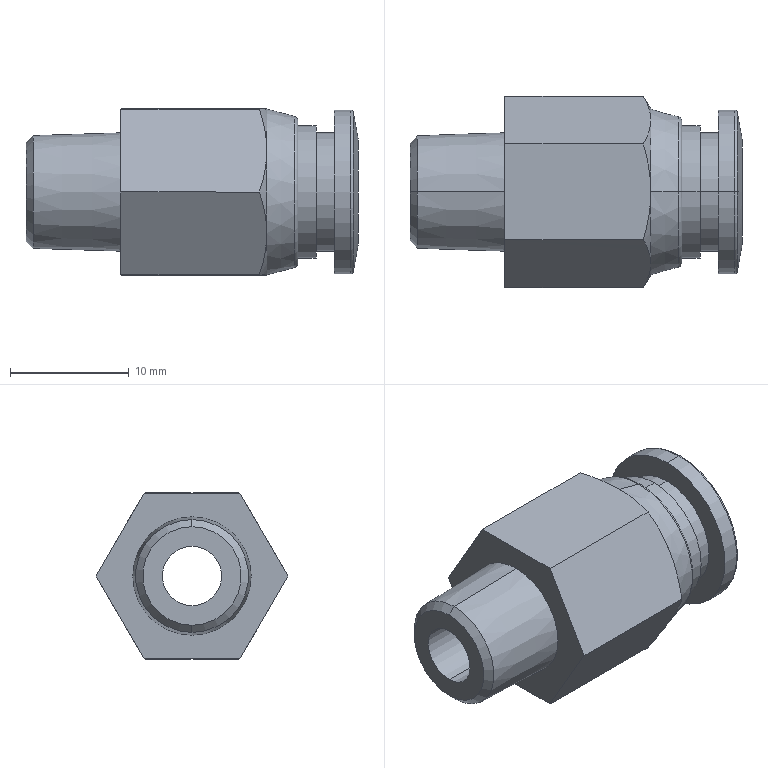Part | SolidWorks | features Fillet 2, BaseBody 1, Chamfer 1, HoleWzd 1, ICE 1, Revolution 1 | 1 solid | 41 faces | box 28 x 16.166 x 14 mm | volume 2490 mm3 | cone 14 | plane 13 | cylinder 10 | torus 4 | commonest cylinder face diameters 5 x2 8 x2 10 x2 11.2 x2 13.8 x2
STEP:
#1=CARTESIAN_POINT('',(22.923,0.,-5.992));
#2=VERTEX_POINT('',#1);
#3=CARTESIAN_POINT('',(22.923,0.,5.992));
#4=VERTEX_POINT('',#3);
#5=CARTESIAN_POINT('',(22.923,0.,0.));
#6=DIRECTION('',(1.,0.,0.));
#7=DIRECTION('',(0.,0.,1.));
#8=AXIS2_PLACEMENT_3D('',#5,#6,#7);
#9=CIRCLE('',#8,5.992);
#10=EDGE_CURVE('',#2,#4,#9,.T.);
#11=ORIENTED_EDGE('',*,*,#10,.F.);
#12=CARTESIAN_POINT('',(22.627,0.,-6.379));
#13=VERTEX_POINT('',#12);
#14=CARTESIAN_POINT('',(22.523,0.,-5.992));
#15=DIRECTION('',(0.,1.,0.));
#16=DIRECTION('',(0.,0.,1.));
#17=AXIS2_PLACEMENT_3D('',#14,#15,#16);
#18=CIRCLE('',#17,0.4);
#19=EDGE_CURVE('',#2,#13,#18,.T.);
#20=ORIENTED_EDGE('',*,*,#19,.T.);
#21=CARTESIAN_POINT('',(22.627,0.,6.379));
#22=VERTEX_POINT('',#21);
#23=CARTESIAN_POINT('',(22.627,0.,0.));
#24=DIRECTION('',(-1.,0.,0.));
#25=DIRECTION('',(0.,0.,1.));
#26=AXIS2_PLACEMENT_3D('',#23,#24,#25);
#27=CIRCLE('',#26,6.379);
#28=EDGE_CURVE('',#22,#13,#27,.T.);
#29=ORIENTED_EDGE('',*,*,#28,.F.);
#30=CARTESIAN_POINT('',(22.523,0.,5.992));
#31=DIRECTION('',(0.,-1.,0.));
#32=DIRECTION('',(1.,0.,0.));
#33=AXIS2_PLACEMENT_3D('',#30,#31,#32);
#34=CIRCLE('',#33,0.4);
#35=EDGE_CURVE('',#4,#22,#34,.T.);
#36=ORIENTED_EDGE('',*,*,#35,.F.);
#37=EDGE_LOOP('',(#11,#20,#29,#36));
#38=FACE_OUTER_BOUND('',#37,.T.);
#39=CARTESIAN_POINT('',(22.523,0.,0.));
#40=DIRECTION('',(-1.,0.,0.));
#41=DIRECTION('',(0.,0.,1.));
#42=AXIS2_PLACEMENT_3D('',#39,#40,#41);
#43=TOROIDAL_SURFACE('',#42,5.992,0.4);
#44=ADVANCED_FACE('',(#38),#43,.T.);
#45=CARTESIAN_POINT('',(27.606,0.,-6.735));
#46=VERTEX_POINT('',#45);
#47=CARTESIAN_POINT('',(27.606,0.,6.735));
#48=VERTEX_POINT('',#47);
#49=CARTESIAN_POINT('',(27.606,0.,0.));
#50=DIRECTION('',(1.,0.,0.));
#51=DIRECTION('',(0.,0.,-1.));
#52=AXIS2_PLACEMENT_3D('',#49,#50,#51);
#53=CIRCLE('',#52,6.735);
#54=EDGE_CURVE('',#46,#48,#53,.T.);
#55=ORIENTED_EDGE('',*,*,#54,.F.);
#56=CARTESIAN_POINT('',(27.409,0.,-6.9));
#57=VERTEX_POINT('',#56);
#58=CARTESIAN_POINT('',(27.409,0.,-6.7));
#59=DIRECTION('',(0.,1.,0.));
#60=DIRECTION('',(0.,0.,1.));
#61=AXIS2_PLACEMENT_3D('',#58,#59,#60);
#62=CIRCLE('',#61,0.2);
#63=EDGE_CURVE('',#46,#57,#62,.T.);
#64=ORIENTED_EDGE('',*,*,#63,.T.);
#65=CARTESIAN_POINT('',(27.409,0.,6.9));
#66=VERTEX_POINT('',#65);
#67=CARTESIAN_POINT('',(27.409,0.,0.));
#68=DIRECTION('',(-1.,0.,0.));
#69=DIRECTION('',(0.,0.,1.));
#70=AXIS2_PLACEMENT_3D('',#67,#68,#69);
#71=CIRCLE('',#70,6.9);
#72=EDGE_CURVE('',#66,#57,#71,.T.);
#73=ORIENTED_EDGE('',*,*,#72,.F.);
#74=CARTESIAN_POINT('',(27.409,0.,6.7));
#75=DIRECTION('',(0.,-1.,0.));
#76=DIRECTION('',(1.,0.,0.));
#77=AXIS2_PLACEMENT_3D('',#74,#75,#76);
#78=CIRCLE('',#77,0.2);
#79=EDGE_CURVE('',#48,#66,#78,.T.);
#80=ORIENTED_EDGE('',*,*,#79,.F.);
#81=EDGE_LOOP('',(#55,#64,#73,#80));
#82=FACE_OUTER_BOUND('',#81,.T.);
#83=CARTESIAN_POINT('',(27.409,0.,0.));
#84=DIRECTION('',(-1.,0.,0.));
#85=DIRECTION('',(0.,0.,1.));
#86=AXIS2_PLACEMENT_3D('',#83,#84,#85);
#87=TOROIDAL_SURFACE('',#86,6.7,0.2);
#88=ADVANCED_FACE('',(#82),#87,.T.);
#89=CARTESIAN_POINT('',(0.,0.,4.158));
#90=VERTEX_POINT('',#89);
#91=CARTESIAN_POINT('',(0.,0.,-4.158));
#92=VERTEX_POINT('',#91);
#93=CARTESIAN_POINT('',(0.,0.,0.));
#94=DIRECTION('',(-1.,0.,0.));
#95=DIRECTION('',(0.,0.,1.));
#96=AXIS2_PLACEMENT_3D('',#93,#94,#95);
#97=CIRCLE('',#96,4.158);
#98=EDGE_CURVE('',#90,#92,#97,.T.);
#99=ORIENTED_EDGE('',*,*,#98,.F.);
#100=CARTESIAN_POINT('',(0.5997,0.,4.758));
#101=VERTEX_POINT('',#100);
#102=CARTESIAN_POINT('',(0.,0.,4.158));
#103=DIRECTION('',(0.7071,0.,0.7071));
#104=VECTOR('',#103,1000.);
#105=LINE('',#102,#104);
#106=EDGE_CURVE('',#90,#101,#105,.T.);
#107=ORIENTED_EDGE('',*,*,#106,.T.);
#108=CARTESIAN_POINT('',(0.5997,0.,-4.758));
#109=VERTEX_POINT('',#108);
#110=CARTESIAN_POINT('',(0.5997,0.,0.));
#111=DIRECTION('',(1.,0.,0.));
#112=DIRECTION('',(0.,0.,1.));
#113=AXIS2_PLACEMENT_3D('',#110,#111,#112);
#114=CIRCLE('',#113,4.758);
#115=EDGE_CURVE('',#109,#101,#114,.T.);
#116=ORIENTED_EDGE('',*,*,#115,.F.);
#117=CARTESIAN_POINT('',(0.,0.,-4.158));
#118=DIRECTION('',(0.7071,0.,-0.7071));
#119=VECTOR('',#118,1000.);
#120=LINE('',#117,#119);
#121=EDGE_CURVE('',#92,#109,#120,.T.);
#122=ORIENTED_EDGE('',*,*,#121,.F.);
#123=EDGE_LOOP('',(#99,#107,#116,#122));
#124=FACE_OUTER_BOUND('',#123,.T.);
#125=CARTESIAN_POINT('',(0.,0.,0.));
#126=DIRECTION('',(1.,0.,0.));
#127=DIRECTION('',(0.,0.,-1.));
#128=AXIS2_PLACEMENT_3D('',#125,#126,#127);
#129=CONICAL_SURFACE('',#128,4.158,0.7854);
#130=ADVANCED_FACE('',(#124),#129,.T.);
#131=CARTESIAN_POINT('',(10.,0.,4.));
#132=VERTEX_POINT('',#131);
#133=CARTESIAN_POINT('',(10.,0.,-4.));
#134=VERTEX_POINT('',#133);
#135=CARTESIAN_POINT('',(10.,0.,0.));
#136=DIRECTION('',(1.,0.,0.));
#137=DIRECTION('',(0.,0.,-1.));
#138=AXIS2_PLACEMENT_3D('',#135,#136,#137);
#139=CIRCLE('',#138,4.);
#140=EDGE_CURVE('',#132,#134,#139,.T.);
#141=ORIENTED_EDGE('',*,*,#140,.F.);
#142=CARTESIAN_POINT('',(28.,0.,4.));
#143=VERTEX_POINT('',#142);
#144=CARTESIAN_POINT('',(28.,0.,4.));
#145=DIRECTION('',(1.,0.,0.));
#146=VECTOR('',#145,1000.);
#147=LINE('',#144,#146);
#148=EDGE_CURVE('',#132,#143,#147,.T.);
#149=ORIENTED_EDGE('',*,*,#148,.T.);
#150=CARTESIAN_POINT('',(28.,0.,-4.));
#151=VERTEX_POINT('',#150);
#152=CARTESIAN_POINT('',(28.,0.,0.));
#153=DIRECTION('',(1.,0.,0.));
#154=DIRECTION('',(0.,0.,-1.));
#155=AXIS2_PLACEMENT_3D('',#152,#153,#154);
#156=CIRCLE('',#155,4.);
#157=EDGE_CURVE('',#143,#151,#156,.T.);
#158=ORIENTED_EDGE('',*,*,#157,.T.);
#159=CARTESIAN_POINT('',(28.,0.,-4.));
#160=DIRECTION('',(1.,0.,0.));
#161=VECTOR('',#160,1000.);
#162=LINE('',#159,#161);
#163=EDGE_CURVE('',#134,#151,#162,.T.);
#164=ORIENTED_EDGE('',*,*,#163,.F.);
#165=EDGE_LOOP('',(#141,#149,#158,#164));
#166=FACE_OUTER_BOUND('',#165,.T.);
#167=CARTESIAN_POINT('',(28.,0.,0.));
#168=DIRECTION('',(1.,0.,0.));
#169=DIRECTION('',(0.,0.,-1.));
#170=AXIS2_PLACEMENT_3D('',#167,#168,#169);
#171=CYLINDRICAL_SURFACE('',#170,4.);
#172=ADVANCED_FACE('',(#166),#171,.F.);
#173=CARTESIAN_POINT('',(0.,0.,2.5));
#174=VERTEX_POINT('',#173);
#175=CARTESIAN_POINT('',(0.,0.,-2.5));
#176=VERTEX_POINT('',#175);
#177=CARTESIAN_POINT('',(0.,0.,0.));
#178=DIRECTION('',(1.,0.,0.));
#179=DIRECTION('',(0.,0.,-1.));
#180=AXIS2_PLACEMENT_3D('',#177,#178,#179);
#181=CIRCLE('',#180,2.5);
#182=EDGE_CURVE('',#174,#176,#181,.T.);
#183=ORIENTED_EDGE('',*,*,#182,.F.);
#184=CARTESIAN_POINT('',(10.,0.,2.5));
#185=VERTEX_POINT('',#184);
#186=CARTESIAN_POINT('',(28.,0.,2.5));
#187=DIRECTION('',(1.,0.,0.));
#188=VECTOR('',#187,1000.);
#189=LINE('',#186,#188);
#190=EDGE_CURVE('',#174,#185,#189,.T.);
#191=ORIENTED_EDGE('',*,*,#190,.T.);
#192=CARTESIAN_POINT('',(10.,0.,-2.5));
#193=VERTEX_POINT('',#192);
#194=CARTESIAN_POINT('',(10.,0.,0.));
#195=DIRECTION('',(1.,0.,0.));
#196=DIRECTION('',(0.,0.,-1.));
#197=AXIS2_PLACEMENT_3D('',#194,#195,#196);
#198=CIRCLE('',#197,2.5);
#199=EDGE_CURVE('',#185,#193,#198,.T.);
#200=ORIENTED_EDGE('',*,*,#199,.T.);
#201=CARTESIAN_POINT('',(28.,0.,-2.5));
#202=DIRECTION('',(1.,0.,0.));
#203=VECTOR('',#202,1000.);
#204=LINE('',#201,#203);
#205=EDGE_CURVE('',#176,#193,#204,.T.);
#206=ORIENTED_EDGE('',*,*,#205,.F.);
#207=EDGE_LOOP('',(#183,#191,#200,#206));
#208=FACE_OUTER_BOUND('',#207,.T.);
#209=CARTESIAN_POINT('',(28.,0.,0.));
#210=DIRECTION('',(1.,0.,0.));
#211=DIRECTION('',(0.,0.,-1.));
#212=AXIS2_PLACEMENT_3D('',#209,#210,#211);
#213=CYLINDRICAL_SURFACE('',#212,2.5);
#214=ADVANCED_FACE('',(#208),#213,.F.);
#215=ORIENTED_EDGE('',*,*,#115,.T.);
#216=CARTESIAN_POINT('',(8.,0.,4.989));
#217=VERTEX_POINT('',#216);
#218=CARTESIAN_POINT('',(0.,0.,4.739));
#219=DIRECTION('',(0.9995,0.,0.0312));
#220=VECTOR('',#219,1000.);
#221=LINE('',#218,#220);
#222=EDGE_CURVE('',#101,#217,#221,.T.);
#223=ORIENTED_EDGE('',*,*,#222,.T.);
#224=CARTESIAN_POINT('',(8.,0.,-4.989));
#225=VERTEX_POINT('',#224);
#226=CARTESIAN_POINT('',(8.,0.,0.));
#227=DIRECTION('',(-1.,0.,0.));
#228=DIRECTION('',(0.,0.,1.));
#229=AXIS2_PLACEMENT_3D('',#226,#227,#228);
#230=CIRCLE('',#229,4.989);
#231=EDGE_CURVE('',#217,#225,#230,.T.);
#232=ORIENTED_EDGE('',*,*,#231,.T.);
#233=CARTESIAN_POINT('',(0.,0.,-4.739));
#234=DIRECTION('',(0.9995,0.,-0.0312));
#235=VECTOR('',#234,1000.);
#236=LINE('',#233,#235);
#237=EDGE_CURVE('',#109,#225,#236,.T.);
#238=ORIENTED_EDGE('',*,*,#237,.F.);
#239=EDGE_LOOP('',(#215,#223,#232,#238));
#240=FACE_OUTER_BOUND('',#239,.T.);
#241=CARTESIAN_POINT('',(0.,0.,0.));
#242=DIRECTION('',(1.,0.,0.));
#243=DIRECTION('',(0.,0.,-1.));
#244=AXIS2_PLACEMENT_3D('',#241,#242,#243);
#245=CONICAL_SURFACE('',#244,4.739,0.03121);
#246=ADVANCED_FACE('',(#240),#245,.T.);
#247=CARTESIAN_POINT('',(28.,0.,4.5));
#248=VERTEX_POINT('',#247);
#249=CARTESIAN_POINT('',(28.,0.,-4.5));
#250=VERTEX_POINT('',#249);
#251=CARTESIAN_POINT('',(28.,0.,0.));
#252=DIRECTION('',(-1.,0.,0.));
#253=DIRECTION('',(0.,0.,1.));
#254=AXIS2_PLACEMENT_3D('',#251,#252,#253);
#255=CIRCLE('',#254,4.5);
#256=EDGE_CURVE('',#248,#250,#255,.T.);
#257=ORIENTED_EDGE('',*,*,#256,.T.);
#258=CARTESIAN_POINT('',(27.606,0.,-6.735));
#259=DIRECTION('',(-0.1736,0.,-0.9848));
#260=VECTOR('',#259,1000.);
#261=LINE('',#258,#260);
#262=EDGE_CURVE('',#250,#46,#261,.T.);
#263=ORIENTED_EDGE('',*,*,#262,.T.);
#264=ORIENTED_EDGE('',*,*,#54,.T.);
#265=CARTESIAN_POINT('',(27.606,0.,6.735));
#266=DIRECTION('',(-0.1736,0.,0.9848));
#267=VECTOR('',#266,1000.);
#268=LINE('',#265,#267);
#269=EDGE_CURVE('',#248,#48,#268,.T.);
#270=ORIENTED_EDGE('',*,*,#269,.F.);
#271=EDGE_LOOP('',(#257,#263,#264,#270));
#272=FACE_OUTER_BOUND('',#271,.T.);
#273=CARTESIAN_POINT('',(27.606,0.,0.));
#274=DIRECTION('',(-1.,0.,0.));
#275=DIRECTION('',(0.,0.,1.));
#276=AXIS2_PLACEMENT_3D('',#273,#274,#275);
#277=CONICAL_SURFACE('',#276,6.735,1.396);
#278=ADVANCED_FACE('',(#272),#277,.T.);
#279=ORIENTED_EDGE('',*,*,#72,.T.);
#280=CARTESIAN_POINT('',(26.,0.,-6.9));
#281=VERTEX_POINT('',#280);
#282=CARTESIAN_POINT('',(28.,0.,-6.9));
#283=DIRECTION('',(-1.,0.,0.));
#284=VECTOR('',#283,1000.);
#285=LINE('',#282,#284);
#286=EDGE_CURVE('',#57,#281,#285,.T.);
#287=ORIENTED_EDGE('',*,*,#286,.T.);
#288=CARTESIAN_POINT('',(26.,0.,6.9));
#289=VERTEX_POINT('',#288);
#290=CARTESIAN_POINT('',(26.,0.,0.));
#291=DIRECTION('',(1.,0.,0.));
#292=DIRECTION('',(0.,0.,1.));
#293=AXIS2_PLACEMENT_3D('',#290,#291,#292);
#294=CIRCLE('',#293,6.9);
#295=EDGE_CURVE('',#281,#289,#294,.T.);
#296=ORIENTED_EDGE('',*,*,#295,.T.);
#297=CARTESIAN_POINT('',(28.,0.,6.9));
#298=DIRECTION('',(-1.,0.,0.));
#299=VECTOR('',#298,1000.);
#300=LINE('',#297,#299);
#301=EDGE_CURVE('',#66,#289,#300,.T.);
#302=ORIENTED_EDGE('',*,*,#301,.F.);
#303=EDGE_LOOP('',(#279,#287,#296,#302));
#304=FACE_OUTER_BOUND('',#303,.T.);
#305=CARTESIAN_POINT('',(28.,0.,0.));
#306=DIRECTION('',(-1.,0.,0.));
#307=DIRECTION('',(0.,0.,1.));
#308=AXIS2_PLACEMENT_3D('',#305,#306,#307);
#309=CYLINDRICAL_SURFACE('',#308,6.9);
#310=ADVANCED_FACE('',(#304),#309,.T.);
#311=CARTESIAN_POINT('',(26.,0.,5.));
#312=VERTEX_POINT('',#311);
#313=CARTESIAN_POINT('',(26.,0.,-5.));
#314=VERTEX_POINT('',#313);
#315=CARTESIAN_POINT('',(26.,0.,0.));
#316=DIRECTION('',(-1.,0.,0.));
#317=DIRECTION('',(0.,0.,1.));
#318=AXIS2_PLACEMENT_3D('',#315,#316,#317);
#319=CIRCLE('',#318,5.);
#320=EDGE_CURVE('',#312,#314,#319,.T.);
#321=ORIENTED_EDGE('',*,*,#320,.T.);
#322=CARTESIAN_POINT('',(24.462,0.,-5.));
#323=VERTEX_POINT('',#322);
#324=CARTESIAN_POINT('',(28.,0.,-5.));
#325=DIRECTION('',(-1.,0.,0.));
#326=VECTOR('',#325,1000.);
#327=LINE('',#324,#326);
#328=EDGE_CURVE('',#314,#323,#327,.T.);
#329=ORIENTED_EDGE('',*,*,#328,.T.);
#330=CARTESIAN_POINT('',(24.462,0.,5.));
#331=VERTEX_POINT('',#330);
#332=CARTESIAN_POINT('',(24.462,0.,0.));
#333=DIRECTION('',(1.,0.,0.));
#334=DIRECTION('',(0.,0.,1.));
#335=AXIS2_PLACEMENT_3D('',#332,#333,#334);
#336=CIRCLE('',#335,5.);
#337=EDGE_CURVE('',#323,#331,#336,.T.);
#338=ORIENTED_EDGE('',*,*,#337,.T.);
#339=CARTESIAN_POINT('',(28.,0.,5.));
#340=DIRECTION('',(-1.,0.,0.));
#341=VECTOR('',#340,1000.);
#342=LINE('',#339,#341);
#343=EDGE_CURVE('',#312,#331,#342,.T.);
#344=ORIENTED_EDGE('',*,*,#343,.F.);
#345=EDGE_LOOP('',(#321,#329,#338,#344));
#346=FACE_OUTER_BOUND('',#345,.T.);
#347=CARTESIAN_POINT('',(28.,0.,0.));
#348=DIRECTION('',(-1.,0.,0.));
#349=DIRECTION('',(0.,0.,1.));
#350=AXIS2_PLACEMENT_3D('',#347,#348,#349);
#351=CYLINDRICAL_SURFACE('',#350,5.);
#352=ADVANCED_FACE('',(#346),#351,.T.);
#353=CARTESIAN_POINT('',(24.462,0.,5.6));
#354=VERTEX_POINT('',#353);
#355=CARTESIAN_POINT('',(24.462,0.,-5.6));
#356=VERTEX_POINT('',#355);
#357=CARTESIAN_POINT('',(24.462,0.,0.));
#358=DIRECTION('',(-1.,0.,0.));
#359=DIRECTION('',(0.,0.,1.));
#360=AXIS2_PLACEMENT_3D('',#357,#358,#359);
#361=CIRCLE('',#360,5.6);
#362=EDGE_CURVE('',#354,#356,#361,.T.);
#363=ORIENTED_EDGE('',*,*,#362,.T.);
#364=CARTESIAN_POINT('',(22.923,0.,-5.6));
#365=VERTEX_POINT('',#364);
#366=CARTESIAN_POINT('',(28.,0.,-5.6));
#367=DIRECTION('',(-1.,0.,0.));
#368=VECTOR('',#367,1000.);
#369=LINE('',#366,#368);
#370=EDGE_CURVE('',#356,#365,#369,.T.);
#371=ORIENTED_EDGE('',*,*,#370,.T.);
#372=CARTESIAN_POINT('',(22.923,0.,5.6));
#373=VERTEX_POINT('',#372);
#374=CARTESIAN_POINT('',(22.923,0.,0.));
#375=DIRECTION('',(1.,0.,0.));
#376=DIRECTION('',(0.,0.,1.));
#377=AXIS2_PLACEMENT_3D('',#374,#375,#376);
#378=CIRCLE('',#377,5.6);
#379=EDGE_CURVE('',#365,#373,#378,.T.);
#380=ORIENTED_EDGE('',*,*,#379,.T.);
#381=CARTESIAN_POINT('',(28.,0.,5.6));
#382=DIRECTION('',(-1.,0.,0.));
#383=VECTOR('',#382,1000.);
#384=LINE('',#381,#383);
#385=EDGE_CURVE('',#354,#373,#384,.T.);
#386=ORIENTED_EDGE('',*,*,#385,.F.);
#387=EDGE_LOOP('',(#363,#371,#380,#386));
#388=FACE_OUTER_BOUND('',#387,.T.);
#389=CARTESIAN_POINT('',(28.,0.,0.));
#390=DIRECTION('',(-1.,0.,0.));
#391=DIRECTION('',(0.,0.,1.));
#392=AXIS2_PLACEMENT_3D('',#389,#390,#391);
#393=CYLINDRICAL_SURFACE('',#392,5.6);
#394=ADVANCED_FACE('',(#388),#393,.T.);
#395=ORIENTED_EDGE('',*,*,#28,.T.);
#396=CARTESIAN_POINT('',(20.308,0.,-7.));
#397=VERTEX_POINT('',#396);
#398=CARTESIAN_POINT('',(20.308,0.,-7.));
#399=DIRECTION('',(-0.9659,0.,-0.2588));
#400=VECTOR('',#399,1000.);
#401=LINE('',#398,#400);
#402=EDGE_CURVE('',#13,#397,#401,.T.);
#403=ORIENTED_EDGE('',*,*,#402,.T.);
#404=CARTESIAN_POINT('',(20.308,6.062,-3.5));
#405=VERTEX_POINT('',#404);
#406=CARTESIAN_POINT('',(20.308,0.,0.));
#407=DIRECTION('',(-1.,0.,0.));
#408=DIRECTION('',(0.,-1.,0.));
#409=AXIS2_PLACEMENT_3D('',#406,#407,#408);
#410=CIRCLE('',#409,7.);
#411=EDGE_CURVE('',#405,#397,#410,.T.);
#412=ORIENTED_EDGE('',*,*,#411,.F.);
#413=CARTESIAN_POINT('',(20.308,6.062,3.5));
#414=VERTEX_POINT('',#413);
#415=CARTESIAN_POINT('',(20.308,0.,0.));
#416=DIRECTION('',(-1.,0.,0.));
#417=DIRECTION('',(0.,-1.,0.));
#418=AXIS2_PLACEMENT_3D('',#415,#416,#417);
#419=CIRCLE('',#418,7.);
#420=EDGE_CURVE('',#414,#405,#419,.T.);
#421=ORIENTED_EDGE('',*,*,#420,.F.);
#422=CARTESIAN_POINT('',(20.308,0.,7.));
#423=VERTEX_POINT('',#422);
#424=CARTESIAN_POINT('',(20.308,0.,0.));
#425=DIRECTION('',(-1.,0.,0.));
#426=DIRECTION('',(0.,-1.,0.));
#427=AXIS2_PLACEMENT_3D('',#424,#425,#426);
#428=CIRCLE('',#427,7.);
#429=EDGE_CURVE('',#423,#414,#428,.T.);
#430=ORIENTED_EDGE('',*,*,#429,.F.);
#431=CARTESIAN_POINT('',(20.308,0.,7.));
#432=DIRECTION('',(-0.9659,0.,0.2588));
#433=VECTOR('',#432,1000.);
#434=LINE('',#431,#433);
#435=EDGE_CURVE('',#22,#423,#434,.T.);
#436=ORIENTED_EDGE('',*,*,#435,.F.);
#437=EDGE_LOOP('',(#395,#403,#412,#421,#430,#436));
#438=FACE_OUTER_BOUND('',#437,.T.);
#439=CARTESIAN_POINT('',(20.308,0.,0.));
#440=DIRECTION('',(-1.,0.,0.));
#441=DIRECTION('',(0.,0.,1.));
#442=AXIS2_PLACEMENT_3D('',#439,#440,#441);
#443=CONICAL_SURFACE('',#442,7.,0.2618);
#444=ADVANCED_FACE('',(#438),#443,.T.);
#445=CARTESIAN_POINT('',(22.923,0.,0.));
#446=DIRECTION('',(1.,0.,0.));
#447=DIRECTION('',(0.,0.,1.));
#448=AXIS2_PLACEMENT_3D('',#445,#446,#447);
#449=CIRCLE('',#448,5.992);
#450=EDGE_CURVE('',#4,#2,#449,.T.);
#451=ORIENTED_EDGE('',*,*,#450,.T.);
#452=ORIENTED_EDGE('',*,*,#10,.T.);
#453=EDGE_LOOP('',(#451,#452));
#454=FACE_OUTER_BOUND('',#453,.T.);
#455=CARTESIAN_POINT('',(22.923,0.,0.));
#456=DIRECTION('',(1.,0.,0.));
#457=DIRECTION('',(0.,0.,1.));
#458=AXIS2_PLACEMENT_3D('',#455,#456,#457);
#459=CIRCLE('',#458,5.6);
#460=EDGE_CURVE('',#373,#365,#459,.T.);
#461=ORIENTED_EDGE('',*,*,#460,.F.);
#462=ORIENTED_EDGE('',*,*,#379,.F.);
#463=EDGE_LOOP('',(#461,#462));
#464=FACE_BOUND('',#463,.T.);
#465=CARTESIAN_POINT('',(22.923,5.992,0.));
#466=DIRECTION('',(-1.,0.,0.));
#467=DIRECTION('',(0.,0.,1.));
#468=AXIS2_PLACEMENT_3D('',#465,#466,#467);
#469=PLANE('',#468);
#470=ADVANCED_FACE('',(#454,#464),#469,.F.);
#471=CARTESIAN_POINT('',(19.682,4.041,7.));
#472=VERTEX_POINT('',#471);
#473=CARTESIAN_POINT('',(19.682,4.041,7.));
#474=CARTESIAN_POINT('',(19.782,3.697,7.));
#475=CARTESIAN_POINT('',(19.87,3.361,7.));
#476=CARTESIAN_POINT('',(19.984,2.863,7.));
#477=CARTESIAN_POINT('',(20.019,2.698,7.));
#478=CARTESIAN_POINT('',(20.067,2.452,7.));
#479=CARTESIAN_POINT('',(20.09,2.329,7.));
#480=CARTESIAN_POINT('',(20.112,2.206,7.));
#481=CARTESIAN_POINT('',(20.126,2.125,7.));
#482=CARTESIAN_POINT('',(20.132,2.086,7.));
#483=CARTESIAN_POINT('',(20.167,1.872,7.));
#484=CARTESIAN_POINT('',(20.191,1.703,7.));
#485=CARTESIAN_POINT('',(20.222,1.45,7.));
#486=CARTESIAN_POINT('',(20.232,1.365,7.));
#487=CARTESIAN_POINT('',(20.249,1.197,7.));
#488=CARTESIAN_POINT('',(20.257,1.114,7.));
#489=CARTESIAN_POINT('',(20.293,0.6831,7.));
#490=CARTESIAN_POINT('',(20.308,0.3429,7.));
#491=CARTESIAN_POINT('',(20.308,0.,7.));
#492=B_SPLINE_CURVE_WITH_KNOTS('',3,(#473,#474,#475,#476,#477,#478,#479,#480,#481,#482,#483,#484,#485,#486,#487,#488,#489,#490,#491),.UNSPECIFIED.,.F.,.F.,(4,2,2,1,2,2,2,2,2,4),(0.,0.25,0.375,0.4375,0.4687,0.5,0.625,0.6875,0.75,1.),.UNSPECIFIED.);
#493=EDGE_CURVE('',#472,#423,#492,.T.);
#494=ORIENTED_EDGE('',*,*,#493,.T.);
#495=ORIENTED_EDGE('',*,*,#429,.T.);
#496=CARTESIAN_POINT('',(20.308,6.062,3.5));
#497=CARTESIAN_POINT('',(20.308,5.976,3.648));
#498=CARTESIAN_POINT('',(20.304,5.891,3.796));
#499=CARTESIAN_POINT('',(20.293,5.763,4.018));
#500=CARTESIAN_POINT('',(20.289,5.72,4.093));
#501=CARTESIAN_POINT('',(20.278,5.634,4.241));
#502=CARTESIAN_POINT('',(20.271,5.591,4.317));
#503=CARTESIAN_POINT('',(20.25,5.464,4.536));
#504=CARTESIAN_POINT('',(20.233,5.38,4.682));
#505=CARTESIAN_POINT('',(20.201,5.253,4.902));
#506=CARTESIAN_POINT('',(20.184,5.189,5.012));
#507=CARTESIAN_POINT('',(20.166,5.126,5.122));
#508=CARTESIAN_POINT('',(20.153,5.083,5.195));
#509=CARTESIAN_POINT('',(20.146,5.061,5.234));
#510=CARTESIAN_POINT('',(20.033,4.714,5.835));
#511=CARTESIAN_POINT('',(19.881,4.386,6.404));
#512=CARTESIAN_POINT('',(19.682,4.041,7.));
#513=B_SPLINE_CURVE_WITH_KNOTS('',3,(#496,#497,#498,#499,#500,#501,#502,#503,#504,#505,#506,#507,#508,#509,#510,#511,#512),.UNSPECIFIED.,.F.,.F.,(4,2,2,2,2,1,2,2,4),(0.,0.125,0.1875,0.25,0.375,0.4375,0.4687,0.5,1.),.UNSPECIFIED.);
#514=EDGE_CURVE('',#414,#472,#513,.T.);
#515=ORIENTED_EDGE('',*,*,#514,.T.);
#516=EDGE_LOOP('',(#494,#495,#515));
#517=FACE_OUTER_BOUND('',#516,.T.);
#518=CARTESIAN_POINT('',(19.679,0.,0.));
#519=DIRECTION('',(-1.,0.,0.));
#520=DIRECTION('',(0.,0.,1.));
#521=AXIS2_PLACEMENT_3D('',#518,#519,#520);
#522=CONICAL_SURFACE('',#521,8.089,1.047);
#523=ADVANCED_FACE('',(#517),#522,.T.);
#524=CARTESIAN_POINT('',(19.682,-4.041,7.));
#525=VERTEX_POINT('',#524);
#526=CARTESIAN_POINT('',(20.308,-6.062,3.5));
#527=VERTEX_POINT('',#526);
#528=CARTESIAN_POINT('',(19.682,-4.041,7.));
#529=CARTESIAN_POINT('',(19.782,-4.214,6.702));
#530=CARTESIAN_POINT('',(19.87,-4.382,6.41));
#531=CARTESIAN_POINT('',(19.984,-4.631,5.979));
#532=CARTESIAN_POINT('',(20.019,-4.713,5.836));
#533=CARTESIAN_POINT('',(20.067,-4.836,5.623));
#534=CARTESIAN_POINT('',(20.09,-4.898,5.517));
#535=CARTESIAN_POINT('',(20.112,-4.959,5.411));
#536=CARTESIAN_POINT('',(20.126,-5.,5.34));
#537=CARTESIAN_POINT('',(20.132,-5.019,5.306));
#538=CARTESIAN_POINT('',(20.167,-5.126,5.122));
#539=CARTESIAN_POINT('',(20.191,-5.211,4.975));
#540=CARTESIAN_POINT('',(20.222,-5.337,4.755));
#541=CARTESIAN_POINT('',(20.232,-5.38,4.682));
#542=CARTESIAN_POINT('',(20.249,-5.464,4.536));
#543=CARTESIAN_POINT('',(20.257,-5.505,4.465));
#544=CARTESIAN_POINT('',(20.293,-5.721,4.092));
#545=CARTESIAN_POINT('',(20.308,-5.891,3.797));
#546=CARTESIAN_POINT('',(20.308,-6.062,3.5));
#547=B_SPLINE_CURVE_WITH_KNOTS('',3,(#528,#529,#530,#531,#532,#533,#534,#535,#536,#537,#538,#539,#540,#541,#542,#543,#544,#545,#546),.UNSPECIFIED.,.F.,.F.,(4,2,2,1,2,2,2,2,2,4),(0.,0.25,0.375,0.4375,0.4687,0.5,0.625,0.6875,0.75,1.),.UNSPECIFIED.);
#548=EDGE_CURVE('',#525,#527,#547,.T.);
#549=ORIENTED_EDGE('',*,*,#548,.T.);
#550=CARTESIAN_POINT('',(20.308,0.,0.));
#551=DIRECTION('',(-1.,0.,0.));
#552=DIRECTION('',(0.,-1.,0.));
#553=AXIS2_PLACEMENT_3D('',#550,#551,#552);
#554=CIRCLE('',#553,7.);
#555=EDGE_CURVE('',#527,#423,#554,.T.);
#556=ORIENTED_EDGE('',*,*,#555,.T.);
#557=CARTESIAN_POINT('',(20.308,0.,7.));
#558=CARTESIAN_POINT('',(20.308,-0.1714,7.));
#559=CARTESIAN_POINT('',(20.304,-0.3422,7.));
#560=CARTESIAN_POINT('',(20.293,-0.5987,7.));
#561=CARTESIAN_POINT('',(20.289,-0.6842,7.));
#562=CARTESIAN_POINT('',(20.278,-0.8557,7.));
#563=CARTESIAN_POINT('',(20.271,-0.9434,7.));
#564=CARTESIAN_POINT('',(20.25,-1.197,7.));
#565=CARTESIAN_POINT('',(20.233,-1.365,7.));
#566=CARTESIAN_POINT('',(20.201,-1.619,7.));
#567=CARTESIAN_POINT('',(20.184,-1.745,7.));
#568=CARTESIAN_POINT('',(20.166,-1.873,7.));
#569=CARTESIAN_POINT('',(20.153,-1.958,7.));
#570=CARTESIAN_POINT('',(20.146,-2.002,7.));
#571=CARTESIAN_POINT('',(20.033,-2.696,7.));
#572=CARTESIAN_POINT('',(19.881,-3.353,7.));
#573=CARTESIAN_POINT('',(19.682,-4.041,7.));
#574=B_SPLINE_CURVE_WITH_KNOTS('',3,(#557,#558,#559,#560,#561,#562,#563,#564,#565,#566,#567,#568,#569,#570,#571,#572,#573),.UNSPECIFIED.,.F.,.F.,(4,2,2,2,2,1,2,2,4),(0.,0.125,0.1875,0.25,0.375,0.4375,0.4687,0.5,1.),.UNSPECIFIED.);
#575=EDGE_CURVE('',#423,#525,#574,.T.);
#576=ORIENTED_EDGE('',*,*,#575,.T.);
#577=EDGE_LOOP('',(#549,#556,#576));
#578=FACE_OUTER_BOUND('',#577,.T.);
#579=CARTESIAN_POINT('',(19.679,0.,0.));
#580=DIRECTION('',(-1.,0.,0.));
#581=DIRECTION('',(0.,0.,1.));
#582=AXIS2_PLACEMENT_3D('',#579,#580,#581);
#583=CONICAL_SURFACE('',#582,8.089,1.047);
#584=ADVANCED_FACE('',(#578),#583,.T.);
#585=CARTESIAN_POINT('',(20.308,-6.062,-3.5));
#586=VERTEX_POINT('',#585);
#587=CARTESIAN_POINT('',(20.308,0.,0.));
#588=DIRECTION('',(-1.,0.,0.));
#589=DIRECTION('',(0.,-1.,0.));
#590=AXIS2_PLACEMENT_3D('',#587,#588,#589);
#591=CIRCLE('',#590,7.);
#592=EDGE_CURVE('',#586,#527,#591,.T.);
#593=ORIENTED_EDGE('',*,*,#592,.T.);
#594=CARTESIAN_POINT('',(19.682,-8.083,0.));
#595=VERTEX_POINT('',#594);
#596=CARTESIAN_POINT('',(20.308,-6.062,3.5));
#597=CARTESIAN_POINT('',(20.308,-6.148,3.352));
#598=CARTESIAN_POINT('',(20.304,-6.233,3.204));
#599=CARTESIAN_POINT('',(20.293,-6.362,2.982));
#600=CARTESIAN_POINT('',(20.289,-6.404,2.907));
#601=CARTESIAN_POINT('',(20.278,-6.49,2.759));
#602=CARTESIAN_POINT('',(20.271,-6.534,2.683));
#603=CARTESIAN_POINT('',(20.25,-6.661,2.464));
#604=CARTESIAN_POINT('',(20.233,-6.745,2.318));
#605=CARTESIAN_POINT('',(20.201,-6.871,2.098));
#606=CARTESIAN_POINT('',(20.184,-6.935,1.988));
#607=CARTESIAN_POINT('',(20.166,-6.999,1.878));
#608=CARTESIAN_POINT('',(20.153,-7.041,1.804));
#609=CARTESIAN_POINT('',(20.146,-7.063,1.766));
#610=CARTESIAN_POINT('',(20.033,-7.41,1.165));
#611=CARTESIAN_POINT('',(19.881,-7.739,0.5963));
#612=CARTESIAN_POINT('',(19.682,-8.083,0.));
#613=B_SPLINE_CURVE_WITH_KNOTS('',3,(#596,#597,#598,#599,#600,#601,#602,#603,#604,#605,#606,#607,#608,#609,#610,#611,#612),.UNSPECIFIED.,.F.,.F.,(4,2,2,2,2,1,2,2,4),(0.,0.125,0.1875,0.25,0.375,0.4375,0.4687,0.5,1.),.UNSPECIFIED.);
#614=EDGE_CURVE('',#527,#595,#613,.T.);
#615=ORIENTED_EDGE('',*,*,#614,.T.);
#616=CARTESIAN_POINT('',(19.682,-8.083,0.));
#617=CARTESIAN_POINT('',(19.782,-7.911,-0.2981));
#618=CARTESIAN_POINT('',(19.87,-7.742,-0.5895));
#619=CARTESIAN_POINT('',(19.984,-7.493,-1.021));
#620=CARTESIAN_POINT('',(20.019,-7.411,-1.163));
#621=CARTESIAN_POINT('',(20.067,-7.288,-1.377));
#622=CARTESIAN_POINT('',(20.09,-7.227,-1.483));
#623=CARTESIAN_POINT('',(20.112,-7.165,-1.589));
#624=CARTESIAN_POINT('',(20.126,-7.125,-1.66));
#625=CARTESIAN_POINT('',(20.132,-7.105,-1.694));
#626=CARTESIAN_POINT('',(20.167,-6.998,-1.878));
#627=CARTESIAN_POINT('',(20.191,-6.914,-2.025));
#628=CARTESIAN_POINT('',(20.222,-6.787,-2.245));
#629=CARTESIAN_POINT('',(20.232,-6.745,-2.318));
#630=CARTESIAN_POINT('',(20.249,-6.661,-2.464));
#631=CARTESIAN_POINT('',(20.257,-6.619,-2.535));
#632=CARTESIAN_POINT('',(20.293,-6.404,-2.908));
#633=CARTESIAN_POINT('',(20.308,-6.234,-3.203));
#634=CARTESIAN_POINT('',(20.308,-6.062,-3.5));
#635=B_SPLINE_CURVE_WITH_KNOTS('',3,(#616,#617,#618,#619,#620,#621,#622,#623,#624,#625,#626,#627,#628,#629,#630,#631,#632,#633,#634),.UNSPECIFIED.,.F.,.F.,(4,2,2,1,2,2,2,2,2,4),(0.,0.25,0.375,0.4375,0.4687,0.5,0.625,0.6875,0.75,1.),.UNSPECIFIED.);
#636=EDGE_CURVE('',#595,#586,#635,.T.);
#637=ORIENTED_EDGE('',*,*,#636,.T.);
#638=EDGE_LOOP('',(#593,#615,#637));
#639=FACE_OUTER_BOUND('',#638,.T.);
#640=CARTESIAN_POINT('',(19.679,0.,0.));
#641=DIRECTION('',(-1.,0.,0.));
#642=DIRECTION('',(0.,0.,1.));
#643=AXIS2_PLACEMENT_3D('',#640,#641,#642);
#644=CONICAL_SURFACE('',#643,8.089,1.047);
#645=ADVANCED_FACE('',(#639),#644,.T.);
#646=CARTESIAN_POINT('',(20.308,0.,0.));
#647=DIRECTION('',(-1.,0.,0.));
#648=DIRECTION('',(0.,-1.,0.));
#649=AXIS2_PLACEMENT_3D('',#646,#647,#648);
#650=CIRCLE('',#649,7.);
#651=EDGE_CURVE('',#397,#586,#650,.T.);
#652=ORIENTED_EDGE('',*,*,#651,.T.);
#653=CARTESIAN_POINT('',(19.682,-4.041,-7.));
#654=VERTEX_POINT('',#653);
#655=CARTESIAN_POINT('',(20.308,-6.062,-3.5));
#656=CARTESIAN_POINT('',(20.308,-5.976,-3.648));
#657=CARTESIAN_POINT('',(20.304,-5.891,-3.796));
#658=CARTESIAN_POINT('',(20.293,-5.763,-4.018));
#659=CARTESIAN_POINT('',(20.289,-5.72,-4.093));
#660=CARTESIAN_POINT('',(20.278,-5.634,-4.241));
#661=CARTESIAN_POINT('',(20.271,-5.591,-4.317));
#662=CARTESIAN_POINT('',(20.25,-5.464,-4.536));
#663=CARTESIAN_POINT('',(20.233,-5.38,-4.682));
#664=CARTESIAN_POINT('',(20.201,-5.253,-4.902));
#665=CARTESIAN_POINT('',(20.184,-5.189,-5.012));
#666=CARTESIAN_POINT('',(20.166,-5.126,-5.122));
#667=CARTESIAN_POINT('',(20.153,-5.083,-5.195));
#668=CARTESIAN_POINT('',(20.146,-5.061,-5.234));
#669=CARTESIAN_POINT('',(20.033,-4.714,-5.835));
#670=CARTESIAN_POINT('',(19.881,-4.386,-6.404));
#671=CARTESIAN_POINT('',(19.682,-4.041,-7.));
#672=B_SPLINE_CURVE_WITH_KNOTS('',3,(#655,#656,#657,#658,#659,#660,#661,#662,#663,#664,#665,#666,#667,#668,#669,#670,#671),.UNSPECIFIED.,.F.,.F.,(4,2,2,2,2,1,2,2,4),(0.,0.125,0.1875,0.25,0.375,0.4375,0.4688,0.5,1.),.UNSPECIFIED.);
#673=EDGE_CURVE('',#586,#654,#672,.T.);
#674=ORIENTED_EDGE('',*,*,#673,.T.);
#675=CARTESIAN_POINT('',(19.682,-4.041,-7.));
#676=CARTESIAN_POINT('',(19.782,-3.697,-7.));
#677=CARTESIAN_POINT('',(19.87,-3.361,-7.));
#678=CARTESIAN_POINT('',(19.984,-2.863,-7.));
#679=CARTESIAN_POINT('',(20.019,-2.698,-7.));
#680=CARTESIAN_POINT('',(20.067,-2.452,-7.));
#681=CARTESIAN_POINT('',(20.09,-2.329,-7.));
#682=CARTESIAN_POINT('',(20.112,-2.206,-7.));
#683=CARTESIAN_POINT('',(20.126,-2.125,-7.));
#684=CARTESIAN_POINT('',(20.132,-2.086,-7.));
#685=CARTESIAN_POINT('',(20.167,-1.872,-7.));
#686=CARTESIAN_POINT('',(20.191,-1.703,-7.));
#687=CARTESIAN_POINT('',(20.222,-1.45,-7.));
#688=CARTESIAN_POINT('',(20.232,-1.365,-7.));
#689=CARTESIAN_POINT('',(20.249,-1.197,-7.));
#690=CARTESIAN_POINT('',(20.257,-1.114,-7.));
#691=CARTESIAN_POINT('',(20.293,-0.6831,-7.));
#692=CARTESIAN_POINT('',(20.308,-0.3429,-7.));
#693=CARTESIAN_POINT('',(20.308,0.,-7.));
#694=B_SPLINE_CURVE_WITH_KNOTS('',3,(#675,#676,#677,#678,#679,#680,#681,#682,#683,#684,#685,#686,#687,#688,#689,#690,#691,#692,#693),.UNSPECIFIED.,.F.,.F.,(4,2,2,1,2,2,2,2,2,4),(0.,0.25,0.375,0.4375,0.4688,0.5,0.625,0.6875,0.75,1.),.UNSPECIFIED.);
#695=EDGE_CURVE('',#654,#397,#694,.T.);
#696=ORIENTED_EDGE('',*,*,#695,.T.);
#697=EDGE_LOOP('',(#652,#674,#696));
#698=FACE_OUTER_BOUND('',#697,.T.);
#699=CARTESIAN_POINT('',(19.679,0.,0.));
#700=DIRECTION('',(-1.,0.,0.));
#701=DIRECTION('',(0.,0.,1.));
#702=AXIS2_PLACEMENT_3D('',#699,#700,#701);
#703=CONICAL_SURFACE('',#702,8.089,1.047);
#704=ADVANCED_FACE('',(#698),#703,.T.);
#705=ORIENTED_EDGE('',*,*,#411,.T.);
#706=CARTESIAN_POINT('',(19.682,4.041,-7.));
#707=VERTEX_POINT('',#706);
#708=CARTESIAN_POINT('',(20.308,0.,-7.));
#709=CARTESIAN_POINT('',(20.308,0.1714,-7.));
#710=CARTESIAN_POINT('',(20.304,0.3422,-7.));
#711=CARTESIAN_POINT('',(20.293,0.5987,-7.));
#712=CARTESIAN_POINT('',(20.289,0.6842,-7.));
#713=CARTESIAN_POINT('',(20.278,0.8557,-7.));
#714=CARTESIAN_POINT('',(20.271,0.9434,-7.));
#715=CARTESIAN_POINT('',(20.25,1.197,-7.));
#716=CARTESIAN_POINT('',(20.233,1.365,-7.));
#717=CARTESIAN_POINT('',(20.201,1.619,-7.));
#718=CARTESIAN_POINT('',(20.184,1.745,-7.));
#719=CARTESIAN_POINT('',(20.166,1.873,-7.));
#720=CARTESIAN_POINT('',(20.153,1.958,-7.));
#721=CARTESIAN_POINT('',(20.146,2.002,-7.));
#722=CARTESIAN_POINT('',(20.033,2.696,-7.));
#723=CARTESIAN_POINT('',(19.881,3.353,-7.));
#724=CARTESIAN_POINT('',(19.682,4.041,-7.));
#725=B_SPLINE_CURVE_WITH_KNOTS('',3,(#708,#709,#710,#711,#712,#713,#714,#715,#716,#717,#718,#719,#720,#721,#722,#723,#724),.UNSPECIFIED.,.F.,.F.,(4,2,2,2,2,1,2,2,4),(0.,0.125,0.1875,0.25,0.375,0.4375,0.4688,0.5,1.),.UNSPECIFIED.);
#726=EDGE_CURVE('',#397,#707,#725,.T.);
#727=ORIENTED_EDGE('',*,*,#726,.T.);
#728=CARTESIAN_POINT('',(19.682,4.041,-7.));
#729=CARTESIAN_POINT('',(19.782,4.214,-6.702));
#730=CARTESIAN_POINT('',(19.87,4.382,-6.41));
#731=CARTESIAN_POINT('',(19.984,4.631,-5.979));
#732=CARTESIAN_POINT('',(20.019,4.713,-5.836));
#733=CARTESIAN_POINT('',(20.067,4.836,-5.623));
#734=CARTESIAN_POINT('',(20.09,4.898,-5.517));
#735=CARTESIAN_POINT('',(20.112,4.959,-5.411));
#736=CARTESIAN_POINT('',(20.126,5.,-5.34));
#737=CARTESIAN_POINT('',(20.132,5.019,-5.306));
#738=CARTESIAN_POINT('',(20.167,5.126,-5.122));
#739=CARTESIAN_POINT('',(20.191,5.211,-4.975));
#740=CARTESIAN_POINT('',(20.222,5.337,-4.755));
#741=CARTESIAN_POINT('',(20.232,5.38,-4.682));
#742=CARTESIAN_POINT('',(20.249,5.464,-4.536));
#743=CARTESIAN_POINT('',(20.257,5.505,-4.465));
#744=CARTESIAN_POINT('',(20.293,5.721,-4.092));
#745=CARTESIAN_POINT('',(20.308,5.891,-3.797));
#746=CARTESIAN_POINT('',(20.308,6.062,-3.5));
#747=B_SPLINE_CURVE_WITH_KNOTS('',3,(#728,#729,#730,#731,#732,#733,#734,#735,#736,#737,#738,#739,#740,#741,#742,#743,#744,#745,#746),.UNSPECIFIED.,.F.,.F.,(4,2,2,1,2,2,2,2,2,4),(0.,0.25,0.375,0.4375,0.4688,0.5,0.625,0.6875,0.75,1.),.UNSPECIFIED.);
#748=EDGE_CURVE('',#707,#405,#747,.T.);
#749=ORIENTED_EDGE('',*,*,#748,.T.);
#750=EDGE_LOOP('',(#705,#727,#749));
#751=FACE_OUTER_BOUND('',#750,.T.);
#752=CARTESIAN_POINT('',(19.679,0.,0.));
#753=DIRECTION('',(-1.,0.,0.));
#754=DIRECTION('',(0.,0.,1.));
#755=AXIS2_PLACEMENT_3D('',#752,#753,#754);
#756=CONICAL_SURFACE('',#755,8.089,1.047);
#757=ADVANCED_FACE('',(#751),#756,.T.);
#758=CARTESIAN_POINT('',(19.682,8.083,0.));
#759=VERTEX_POINT('',#758);
#760=CARTESIAN_POINT('',(19.682,8.083,0.));
#761=CARTESIAN_POINT('',(19.782,7.911,0.2981));
#762=CARTESIAN_POINT('',(19.87,7.742,0.5895));
#763=CARTESIAN_POINT('',(19.984,7.493,1.021));
#764=CARTESIAN_POINT('',(20.019,7.411,1.163));
#765=CARTESIAN_POINT('',(20.067,7.288,1.377));
#766=CARTESIAN_POINT('',(20.09,7.227,1.483));
#767=CARTESIAN_POINT('',(20.112,7.165,1.589));
#768=CARTESIAN_POINT('',(20.126,7.125,1.66));
#769=CARTESIAN_POINT('',(20.132,7.105,1.694));
#770=CARTESIAN_POINT('',(20.167,6.998,1.878));
#771=CARTESIAN_POINT('',(20.191,6.914,2.025));
#772=CARTESIAN_POINT('',(20.222,6.787,2.245));
#773=CARTESIAN_POINT('',(20.232,6.745,2.318));
#774=CARTESIAN_POINT('',(20.249,6.661,2.464));
#775=CARTESIAN_POINT('',(20.257,6.619,2.535));
#776=CARTESIAN_POINT('',(20.293,6.404,2.908));
#777=CARTESIAN_POINT('',(20.308,6.234,3.203));
#778=CARTESIAN_POINT('',(20.308,6.062,3.5));
#779=B_SPLINE_CURVE_WITH_KNOTS('',3,(#760,#761,#762,#763,#764,#765,#766,#767,#768,#769,#770,#771,#772,#773,#774,#775,#776,#777,#778),.UNSPECIFIED.,.F.,.F.,(4,2,2,1,2,2,2,2,2,4),(0.,0.25,0.375,0.4375,0.4687,0.5,0.625,0.6875,0.75,1.),.UNSPECIFIED.);
#780=EDGE_CURVE('',#759,#414,#779,.T.);
#781=ORIENTED_EDGE('',*,*,#780,.T.);
#782=ORIENTED_EDGE('',*,*,#420,.T.);
#783=CARTESIAN_POINT('',(20.308,6.062,-3.5));
#784=CARTESIAN_POINT('',(20.308,6.148,-3.352));
#785=CARTESIAN_POINT('',(20.304,6.233,-3.204));
#786=CARTESIAN_POINT('',(20.293,6.362,-2.982));
#787=CARTESIAN_POINT('',(20.289,6.404,-2.907));
#788=CARTESIAN_POINT('',(20.278,6.49,-2.759));
#789=CARTESIAN_POINT('',(20.271,6.534,-2.683));
#790=CARTESIAN_POINT('',(20.25,6.661,-2.464));
#791=CARTESIAN_POINT('',(20.233,6.745,-2.318));
#792=CARTESIAN_POINT('',(20.201,6.871,-2.098));
#793=CARTESIAN_POINT('',(20.184,6.935,-1.988));
#794=CARTESIAN_POINT('',(20.166,6.999,-1.878));
#795=CARTESIAN_POINT('',(20.153,7.041,-1.804));
#796=CARTESIAN_POINT('',(20.146,7.063,-1.766));
#797=CARTESIAN_POINT('',(20.033,7.41,-1.165));
#798=CARTESIAN_POINT('',(19.881,7.739,-0.5963));
#799=CARTESIAN_POINT('',(19.682,8.083,0.));
#800=B_SPLINE_CURVE_WITH_KNOTS('',3,(#783,#784,#785,#786,#787,#788,#789,#790,#791,#792,#793,#794,#795,#796,#797,#798,#799),.UNSPECIFIED.,.F.,.F.,(4,2,2,2,2,1,2,2,4),(0.,0.125,0.1875,0.25,0.375,0.4375,0.4687,0.5,1.),.UNSPECIFIED.);
#801=EDGE_CURVE('',#405,#759,#800,.T.);
#802=ORIENTED_EDGE('',*,*,#801,.T.);
#803=EDGE_LOOP('',(#781,#782,#802));
#804=FACE_OUTER_BOUND('',#803,.T.);
#805=CARTESIAN_POINT('',(19.679,0.,0.));
#806=DIRECTION('',(-1.,0.,0.));
#807=DIRECTION('',(0.,-1.,0.));
#808=AXIS2_PLACEMENT_3D('',#805,#806,#807);
#809=CONICAL_SURFACE('',#808,8.089,1.047);
#810=ADVANCED_FACE('',(#804),#809,.T.);
#811=ORIENTED_EDGE('',*,*,#780,.F.);
#812=CARTESIAN_POINT('',(8.,8.083,0.));
#813=VERTEX_POINT('',#812);
#814=CARTESIAN_POINT('',(8.,8.083,0.));
#815=DIRECTION('',(1.,0.,0.));
#816=VECTOR('',#815,1000.);
#817=LINE('',#814,#816);
#818=EDGE_CURVE('',#813,#759,#817,.T.);
#819=ORIENTED_EDGE('',*,*,#818,.F.);
#820=CARTESIAN_POINT('',(8.,4.041,7.));
#821=VERTEX_POINT('',#820);
#822=CARTESIAN_POINT('',(8.,8.083,0.));
#823=DIRECTION('',(0.,0.5,-0.866));
#824=VECTOR('',#823,1000.);
#825=LINE('',#822,#824);
#826=EDGE_CURVE('',#821,#813,#825,.T.);
#827=ORIENTED_EDGE('',*,*,#826,.F.);
#828=CARTESIAN_POINT('',(8.,4.041,7.));
#829=DIRECTION('',(1.,0.,0.));
#830=VECTOR('',#829,1000.);
#831=LINE('',#828,#830);
#832=EDGE_CURVE('',#821,#472,#831,.T.);
#833=ORIENTED_EDGE('',*,*,#832,.T.);
#834=ORIENTED_EDGE('',*,*,#514,.F.);
#835=EDGE_LOOP('',(#811,#819,#827,#833,#834));
#836=FACE_OUTER_BOUND('',#835,.T.);
#837=CARTESIAN_POINT('',(20.308,8.083,0.));
#838=DIRECTION('',(0.,-0.866,-0.5));
#839=DIRECTION('',(0.,0.5,-0.866));
#840=AXIS2_PLACEMENT_3D('',#837,#838,#839);
#841=PLANE('',#840);
#842=ADVANCED_FACE('',(#836),#841,.F.);
#843=ORIENTED_EDGE('',*,*,#493,.F.);
#844=ORIENTED_EDGE('',*,*,#832,.F.);
#845=CARTESIAN_POINT('',(8.,-4.041,7.));
#846=VERTEX_POINT('',#845);
#847=CARTESIAN_POINT('',(8.,4.041,7.));
#848=DIRECTION('',(0.,1.,0.));
#849=VECTOR('',#848,1000.);
#850=LINE('',#847,#849);
#851=EDGE_CURVE('',#846,#821,#850,.T.);
#852=ORIENTED_EDGE('',*,*,#851,.F.);
#853=CARTESIAN_POINT('',(8.,-4.041,7.));
#854=DIRECTION('',(1.,0.,0.));
#855=VECTOR('',#854,1000.);
#856=LINE('',#853,#855);
#857=EDGE_CURVE('',#846,#525,#856,.T.);
#858=ORIENTED_EDGE('',*,*,#857,.T.);
#859=ORIENTED_EDGE('',*,*,#575,.F.);
#860=EDGE_LOOP('',(#843,#844,#852,#858,#859));
#861=FACE_OUTER_BOUND('',#860,.T.);
#862=CARTESIAN_POINT('',(20.308,4.041,7.));
#863=DIRECTION('',(0.,0.,-1.));
#864=DIRECTION('',(0.,-1.,0.));
#865=AXIS2_PLACEMENT_3D('',#862,#863,#864);
#866=PLANE('',#865);
#867=ADVANCED_FACE('',(#861),#866,.F.);
#868=ORIENTED_EDGE('',*,*,#548,.F.);
#869=ORIENTED_EDGE('',*,*,#857,.F.);
#870=CARTESIAN_POINT('',(8.,-8.083,0.));
#871=VERTEX_POINT('',#870);
#872=CARTESIAN_POINT('',(8.,-4.041,7.));
#873=DIRECTION('',(0.,0.5,0.866));
#874=VECTOR('',#873,1000.);
#875=LINE('',#872,#874);
#876=EDGE_CURVE('',#871,#846,#875,.T.);
#877=ORIENTED_EDGE('',*,*,#876,.F.);
#878=CARTESIAN_POINT('',(8.,-8.083,0.));
#879=DIRECTION('',(1.,0.,0.));
#880=VECTOR('',#879,1000.);
#881=LINE('',#878,#880);
#882=EDGE_CURVE('',#871,#595,#881,.T.);
#883=ORIENTED_EDGE('',*,*,#882,.T.);
#884=ORIENTED_EDGE('',*,*,#614,.F.);
#885=EDGE_LOOP('',(#868,#869,#877,#883,#884));
#886=FACE_OUTER_BOUND('',#885,.T.);
#887=CARTESIAN_POINT('',(20.308,-4.041,7.));
#888=DIRECTION('',(0.,0.866,-0.5));
#889=DIRECTION('',(-1.,0.,0.));
#890=AXIS2_PLACEMENT_3D('',#887,#888,#889);
#891=PLANE('',#890);
#892=ADVANCED_FACE('',(#886),#891,.F.);
#893=ORIENTED_EDGE('',*,*,#636,.F.);
#894=ORIENTED_EDGE('',*,*,#882,.F.);
#895=CARTESIAN_POINT('',(8.,-4.041,-7.));
#896=VERTEX_POINT('',#895);
#897=CARTESIAN_POINT('',(8.,-8.083,0.));
#898=DIRECTION('',(0.,-0.5,0.866));
#899=VECTOR('',#898,1000.);
#900=LINE('',#897,#899);
#901=EDGE_CURVE('',#896,#871,#900,.T.);
#902=ORIENTED_EDGE('',*,*,#901,.F.);
#903=CARTESIAN_POINT('',(8.,-4.041,-7.));
#904=DIRECTION('',(1.,0.,0.));
#905=VECTOR('',#904,1000.);
#906=LINE('',#903,#905);
#907=EDGE_CURVE('',#896,#654,#906,.T.);
#908=ORIENTED_EDGE('',*,*,#907,.T.);
#909=ORIENTED_EDGE('',*,*,#673,.F.);
#910=EDGE_LOOP('',(#893,#894,#902,#908,#909));
#911=FACE_OUTER_BOUND('',#910,.T.);
#912=CARTESIAN_POINT('',(20.308,-8.083,0.));
#913=DIRECTION('',(0.,0.866,0.5));
#914=DIRECTION('',(1.,0.,0.));
#915=AXIS2_PLACEMENT_3D('',#912,#913,#914);
#916=PLANE('',#915);
#917=ADVANCED_FACE('',(#911),#916,.F.);
#918=ORIENTED_EDGE('',*,*,#695,.F.);
#919=ORIENTED_EDGE('',*,*,#907,.F.);
#920=CARTESIAN_POINT('',(8.,4.041,-7.));
#921=VERTEX_POINT('',#920);
#922=CARTESIAN_POINT('',(8.,-4.041,-7.));
#923=DIRECTION('',(0.,-1.,0.));
#924=VECTOR('',#923,1000.);
#925=LINE('',#922,#924);
#926=EDGE_CURVE('',#921,#896,#925,.T.);
#927=ORIENTED_EDGE('',*,*,#926,.F.);
#928=CARTESIAN_POINT('',(8.,4.041,-7.));
#929=DIRECTION('',(1.,0.,0.));
#930=VECTOR('',#929,1000.);
#931=LINE('',#928,#930);
#932=EDGE_CURVE('',#921,#707,#931,.T.);
#933=ORIENTED_EDGE('',*,*,#932,.T.);
#934=ORIENTED_EDGE('',*,*,#726,.F.);
#935=EDGE_LOOP('',(#918,#919,#927,#933,#934));
#936=FACE_OUTER_BOUND('',#935,.T.);
#937=CARTESIAN_POINT('',(20.308,-4.041,-7.));
#938=DIRECTION('',(0.,0.,1.));
#939=DIRECTION('',(1.,0.,0.));
#940=AXIS2_PLACEMENT_3D('',#937,#938,#939);
#941=PLANE('',#940);
#942=ADVANCED_FACE('',(#936),#941,.F.);
#943=ORIENTED_EDGE('',*,*,#748,.F.);
#944=ORIENTED_EDGE('',*,*,#932,.F.);
#945=CARTESIAN_POINT('',(8.,4.041,-7.));
#946=DIRECTION('',(0.,-0.5,-0.866));
#947=VECTOR('',#946,1000.);
#948=LINE('',#945,#947);
#949=EDGE_CURVE('',#813,#921,#948,.T.);
#950=ORIENTED_EDGE('',*,*,#949,.F.);
#951=ORIENTED_EDGE('',*,*,#818,.T.);
#952=ORIENTED_EDGE('',*,*,#801,.F.);
#953=EDGE_LOOP('',(#943,#944,#950,#951,#952));
#954=FACE_OUTER_BOUND('',#953,.T.);
#955=CARTESIAN_POINT('',(20.308,4.041,-7.));
#956=DIRECTION('',(0.,-0.866,0.5));
#957=DIRECTION('',(-1.,0.,0.));
#958=AXIS2_PLACEMENT_3D('',#955,#956,#957);
#959=PLANE('',#958);
#960=ADVANCED_FACE('',(#954),#959,.F.);
#961=CARTESIAN_POINT('',(24.462,0.,0.));
#962=DIRECTION('',(1.,0.,0.));
#963=DIRECTION('',(0.,0.,1.));
#964=AXIS2_PLACEMENT_3D('',#961,#962,#963);
#965=CIRCLE('',#964,5.);
#966=EDGE_CURVE('',#331,#323,#965,.T.);
#967=ORIENTED_EDGE('',*,*,#966,.F.);
#968=ORIENTED_EDGE('',*,*,#337,.F.);
#969=EDGE_LOOP('',(#967,#968));
#970=FACE_BOUND('',#969,.T.);
#971=ORIENTED_EDGE('',*,*,#362,.F.);
#972=CARTESIAN_POINT('',(24.462,0.,0.));
#973=DIRECTION('',(-1.,0.,0.));
#974=DIRECTION('',(0.,0.,1.));
#975=AXIS2_PLACEMENT_3D('',#972,#973,#974);
#976=CIRCLE('',#975,5.6);
#977=EDGE_CURVE('',#356,#354,#976,.T.);
#978=ORIENTED_EDGE('',*,*,#977,.F.);
#979=EDGE_LOOP('',(#971,#978));
#980=FACE_OUTER_BOUND('',#979,.T.);
#981=CARTESIAN_POINT('',(24.462,5.6,0.));
#982=DIRECTION('',(-1.,0.,0.));
#983=DIRECTION('',(0.,0.,1.));
#984=AXIS2_PLACEMENT_3D('',#981,#982,#983);
#985=PLANE('',#984);
#986=ADVANCED_FACE('',(#970,#980),#985,.F.);
#987=ORIENTED_EDGE('',*,*,#320,.F.);
#988=CARTESIAN_POINT('',(26.,0.,0.));
#989=DIRECTION('',(-1.,0.,0.));
#990=DIRECTION('',(0.,0.,1.));
#991=AXIS2_PLACEMENT_3D('',#988,#989,#990);
#992=CIRCLE('',#991,5.);
#993=EDGE_CURVE('',#314,#312,#992,.T.);
#994=ORIENTED_EDGE('',*,*,#993,.F.);
#995=EDGE_LOOP('',(#987,#994));
#996=FACE_BOUND('',#995,.T.);
#997=CARTESIAN_POINT('',(26.,0.,0.));
#998=DIRECTION('',(1.,0.,0.));
#999=DIRECTION('',(0.,0.,1.));
#1000=AXIS2_PLACEMENT_3D('',#997,#998,#999);
#1001=CIRCLE('',#1000,6.9);
#1002=EDGE_CURVE('',#289,#281,#1001,.T.);
#1003=ORIENTED_EDGE('',*,*,#1002,.F.);
#1004=ORIENTED_EDGE('',*,*,#295,.F.);
#1005=EDGE_LOOP('',(#1003,#1004));
#1006=FACE_OUTER_BOUND('',#1005,.T.);
#1007=CARTESIAN_POINT('',(26.,5.,0.));
#1008=DIRECTION('',(1.,0.,0.));
#1009=DIRECTION('',(0.,1.,0.));
#1010=AXIS2_PLACEMENT_3D('',#1007,#1008,#1009);
#1011=PLANE('',#1010);
#1012=ADVANCED_FACE('',(#996,#1006),#1011,.F.);
#1013=CARTESIAN_POINT('',(28.,0.,0.));
#1014=DIRECTION('',(1.,0.,0.));
#1015=DIRECTION('',(0.,0.,-1.));
#1016=AXIS2_PLACEMENT_3D('',#1013,#1014,#1015);
#1017=CIRCLE('',#1016,4.);
#1018=EDGE_CURVE('',#151,#143,#1017,.T.);
#1019=ORIENTED_EDGE('',*,*,#1018,.F.);
#1020=ORIENTED_EDGE('',*,*,#157,.F.);
#1021=EDGE_LOOP('',(#1019,#1020));
#1022=FACE_BOUND('',#1021,.T.);
#1023=ORIENTED_EDGE('',*,*,#256,.F.);
#1024=CARTESIAN_POINT('',(28.,0.,0.));
#1025=DIRECTION('',(-1.,0.,0.));
#1026=DIRECTION('',(0.,0.,1.));
#1027=AXIS2_PLACEMENT_3D('',#1024,#1025,#1026);
#1028=CIRCLE('',#1027,4.5);
#1029=EDGE_CURVE('',#250,#248,#1028,.T.);
#1030=ORIENTED_EDGE('',*,*,#1029,.F.);
#1031=EDGE_LOOP('',(#1023,#1030));
#1032=FACE_OUTER_BOUND('',#1031,.T.);
#1033=CARTESIAN_POINT('',(28.,4.5,0.));
#1034=DIRECTION('',(-1.,0.,0.));
#1035=DIRECTION('',(0.,0.,1.));
#1036=AXIS2_PLACEMENT_3D('',#1033,#1034,#1035);
#1037=PLANE('',#1036);
#1038=ADVANCED_FACE('',(#1022,#1032),#1037,.F.);
#1039=ORIENTED_EDGE('',*,*,#402,.F.);
#1040=CARTESIAN_POINT('',(22.627,0.,0.));
#1041=DIRECTION('',(-1.,0.,0.));
#1042=DIRECTION('',(0.,0.,1.));
#1043=AXIS2_PLACEMENT_3D('',#1040,#1041,#1042);
#1044=CIRCLE('',#1043,6.379);
#1045=EDGE_CURVE('',#13,#22,#1044,.T.);
#1046=ORIENTED_EDGE('',*,*,#1045,.T.);
#1047=ORIENTED_EDGE('',*,*,#435,.T.);
#1048=ORIENTED_EDGE('',*,*,#555,.F.);
#1049=ORIENTED_EDGE('',*,*,#592,.F.);
#1050=ORIENTED_EDGE('',*,*,#651,.F.);
#1051=EDGE_LOOP('',(#1039,#1046,#1047,#1048,#1049,#1050));
#1052=FACE_OUTER_BOUND('',#1051,.T.);
#1053=CARTESIAN_POINT('',(20.308,0.,0.));
#1054=DIRECTION('',(-1.,0.,0.));
#1055=DIRECTION('',(0.,0.,1.));
#1056=AXIS2_PLACEMENT_3D('',#1053,#1054,#1055);
#1057=CONICAL_SURFACE('',#1056,7.,0.2618);
#1058=ADVANCED_FACE('',(#1052),#1057,.T.);
#1059=ORIENTED_EDGE('',*,*,#370,.F.);
#1060=ORIENTED_EDGE('',*,*,#977,.T.);
#1061=ORIENTED_EDGE('',*,*,#385,.T.);
#1062=ORIENTED_EDGE('',*,*,#460,.T.);
#1063=EDGE_LOOP('',(#1059,#1060,#1061,#1062));
#1064=FACE_OUTER_BOUND('',#1063,.T.);
#1065=CARTESIAN_POINT('',(28.,0.,0.));
#1066=DIRECTION('',(-1.,0.,0.));
#1067=DIRECTION('',(0.,0.,1.));
#1068=AXIS2_PLACEMENT_3D('',#1065,#1066,#1067);
#1069=CYLINDRICAL_SURFACE('',#1068,5.6);
#1070=ADVANCED_FACE('',(#1064),#1069,.T.);
#1071=ORIENTED_EDGE('',*,*,#328,.F.);
#1072=ORIENTED_EDGE('',*,*,#993,.T.);
#1073=ORIENTED_EDGE('',*,*,#343,.T.);
#1074=ORIENTED_EDGE('',*,*,#966,.T.);
#1075=EDGE_LOOP('',(#1071,#1072,#1073,#1074));
#1076=FACE_OUTER_BOUND('',#1075,.T.);
#1077=CARTESIAN_POINT('',(28.,0.,0.));
#1078=DIRECTION('',(-1.,0.,0.));
#1079=DIRECTION('',(0.,0.,1.));
#1080=AXIS2_PLACEMENT_3D('',#1077,#1078,#1079);
#1081=CYLINDRICAL_SURFACE('',#1080,5.);
#1082=ADVANCED_FACE('',(#1076),#1081,.T.);
#1083=ORIENTED_EDGE('',*,*,#286,.F.);
#1084=CARTESIAN_POINT('',(27.409,0.,0.));
#1085=DIRECTION('',(-1.,0.,0.));
#1086=DIRECTION('',(0.,0.,1.));
#1087=AXIS2_PLACEMENT_3D('',#1084,#1085,#1086);
#1088=CIRCLE('',#1087,6.9);
#1089=EDGE_CURVE('',#57,#66,#1088,.T.);
#1090=ORIENTED_EDGE('',*,*,#1089,.T.);
#1091=ORIENTED_EDGE('',*,*,#301,.T.);
#1092=ORIENTED_EDGE('',*,*,#1002,.T.);
#1093=EDGE_LOOP('',(#1083,#1090,#1091,#1092));
#1094=FACE_OUTER_BOUND('',#1093,.T.);
#1095=CARTESIAN_POINT('',(28.,0.,0.));
#1096=DIRECTION('',(-1.,0.,0.));
#1097=DIRECTION('',(0.,0.,1.));
#1098=AXIS2_PLACEMENT_3D('',#1095,#1096,#1097);
#1099=CYLINDRICAL_SURFACE('',#1098,6.9);
#1100=ADVANCED_FACE('',(#1094),#1099,.T.);
#1101=ORIENTED_EDGE('',*,*,#262,.F.);
#1102=ORIENTED_EDGE('',*,*,#1029,.T.);
#1103=ORIENTED_EDGE('',*,*,#269,.T.);
#1104=CARTESIAN_POINT('',(27.606,0.,0.));
#1105=DIRECTION('',(1.,0.,0.));
#1106=DIRECTION('',(0.,0.,-1.));
#1107=AXIS2_PLACEMENT_3D('',#1104,#1105,#1106);
#1108=CIRCLE('',#1107,6.735);
#1109=EDGE_CURVE('',#48,#46,#1108,.T.);
#1110=ORIENTED_EDGE('',*,*,#1109,.T.);
#1111=EDGE_LOOP('',(#1101,#1102,#1103,#1110));
#1112=FACE_OUTER_BOUND('',#1111,.T.);
#1113=CARTESIAN_POINT('',(27.606,0.,0.));
#1114=DIRECTION('',(-1.,0.,0.));
#1115=DIRECTION('',(0.,0.,1.));
#1116=AXIS2_PLACEMENT_3D('',#1113,#1114,#1115);
#1117=CONICAL_SURFACE('',#1116,6.735,1.396);
#1118=ADVANCED_FACE('',(#1112),#1117,.T.);
#1119=CARTESIAN_POINT('',(8.,0.,0.));
#1120=DIRECTION('',(-1.,0.,0.));
#1121=DIRECTION('',(0.,0.,1.));
#1122=AXIS2_PLACEMENT_3D('',#1119,#1120,#1121);
#1123=CIRCLE('',#1122,4.989);
#1124=EDGE_CURVE('',#225,#217,#1123,.T.);
#1125=ORIENTED_EDGE('',*,*,#1124,.F.);
#1126=ORIENTED_EDGE('',*,*,#231,.F.);
#1127=EDGE_LOOP('',(#1125,#1126));
#1128=FACE_BOUND('',#1127,.T.);
#1129=ORIENTED_EDGE('',*,*,#901,.T.);
#1130=ORIENTED_EDGE('',*,*,#876,.T.);
#1131=ORIENTED_EDGE('',*,*,#851,.T.);
#1132=ORIENTED_EDGE('',*,*,#826,.T.);
#1133=ORIENTED_EDGE('',*,*,#949,.T.);
#1134=ORIENTED_EDGE('',*,*,#926,.T.);
#1135=EDGE_LOOP('',(#1129,#1130,#1131,#1132,#1133,#1134));
#1136=FACE_OUTER_BOUND('',#1135,.T.);
#1137=CARTESIAN_POINT('',(8.,0.,0.));
#1138=DIRECTION('',(1.,0.,0.));
#1139=DIRECTION('',(0.,0.,-1.));
#1140=AXIS2_PLACEMENT_3D('',#1137,#1138,#1139);
#1141=PLANE('',#1140);
#1142=ADVANCED_FACE('',(#1128,#1136),#1141,.F.);
#1143=ORIENTED_EDGE('',*,*,#222,.F.);
#1144=CARTESIAN_POINT('',(0.5997,0.,0.));
#1145=DIRECTION('',(1.,0.,0.));
#1146=DIRECTION('',(0.,0.,1.));
#1147=AXIS2_PLACEMENT_3D('',#1144,#1145,#1146);
#1148=CIRCLE('',#1147,4.758);
#1149=EDGE_CURVE('',#101,#109,#1148,.T.);
#1150=ORIENTED_EDGE('',*,*,#1149,.T.);
#1151=ORIENTED_EDGE('',*,*,#237,.T.);
#1152=ORIENTED_EDGE('',*,*,#1124,.T.);
#1153=EDGE_LOOP('',(#1143,#1150,#1151,#1152));
#1154=FACE_OUTER_BOUND('',#1153,.T.);
#1155=CARTESIAN_POINT('',(0.,0.,0.));
#1156=DIRECTION('',(1.,0.,0.));
#1157=DIRECTION('',(0.,0.,-1.));
#1158=AXIS2_PLACEMENT_3D('',#1155,#1156,#1157);
#1159=CONICAL_SURFACE('',#1158,4.739,0.03121);
#1160=ADVANCED_FACE('',(#1154),#1159,.T.);
#1161=CARTESIAN_POINT('',(0.,0.,0.));
#1162=DIRECTION('',(-1.,0.,0.));
#1163=DIRECTION('',(0.,0.,1.));
#1164=AXIS2_PLACEMENT_3D('',#1161,#1162,#1163);
#1165=CIRCLE('',#1164,4.158);
#1166=EDGE_CURVE('',#92,#90,#1165,.T.);
#1167=ORIENTED_EDGE('',*,*,#1166,.T.);
#1168=ORIENTED_EDGE('',*,*,#98,.T.);
#1169=EDGE_LOOP('',(#1167,#1168));
#1170=FACE_OUTER_BOUND('',#1169,.T.);
#1171=CARTESIAN_POINT('',(0.,0.,0.));
#1172=DIRECTION('',(1.,0.,0.));
#1173=DIRECTION('',(0.,0.,-1.));
#1174=AXIS2_PLACEMENT_3D('',#1171,#1172,#1173);
#1175=CIRCLE('',#1174,2.5);
#1176=EDGE_CURVE('',#176,#174,#1175,.T.);
#1177=ORIENTED_EDGE('',*,*,#1176,.T.);
#1178=ORIENTED_EDGE('',*,*,#182,.T.);
#1179=EDGE_LOOP('',(#1177,#1178));
#1180=FACE_BOUND('',#1179,.T.);
#1181=CARTESIAN_POINT('',(0.,0.,0.));
#1182=DIRECTION('',(-1.,0.,0.));
#1183=DIRECTION('',(0.,0.,1.));
#1184=AXIS2_PLACEMENT_3D('',#1181,#1182,#1183);
#1185=PLANE('',#1184);
#1186=ADVANCED_FACE('',(#1170,#1180),#1185,.T.);
#1187=ORIENTED_EDGE('',*,*,#190,.F.);
#1188=ORIENTED_EDGE('',*,*,#1176,.F.);
#1189=ORIENTED_EDGE('',*,*,#205,.T.);
#1190=CARTESIAN_POINT('',(10.,0.,0.));
#1191=DIRECTION('',(1.,0.,0.));
#1192=DIRECTION('',(0.,0.,-1.));
#1193=AXIS2_PLACEMENT_3D('',#1190,#1191,#1192);
#1194=CIRCLE('',#1193,2.5);
#1195=EDGE_CURVE('',#193,#185,#1194,.T.);
#1196=ORIENTED_EDGE('',*,*,#1195,.T.);
#1197=EDGE_LOOP('',(#1187,#1188,#1189,#1196));
#1198=FACE_OUTER_BOUND('',#1197,.T.);
#1199=CARTESIAN_POINT('',(28.,0.,0.));
#1200=DIRECTION('',(1.,0.,0.));
#1201=DIRECTION('',(0.,0.,-1.));
#1202=AXIS2_PLACEMENT_3D('',#1199,#1200,#1201);
#1203=CYLINDRICAL_SURFACE('',#1202,2.5);
#1204=ADVANCED_FACE('',(#1198),#1203,.F.);
#1205=ORIENTED_EDGE('',*,*,#1195,.F.);
#1206=ORIENTED_EDGE('',*,*,#199,.F.);
#1207=EDGE_LOOP('',(#1205,#1206));
#1208=FACE_BOUND('',#1207,.T.);
#1209=CARTESIAN_POINT('',(10.,0.,0.));
#1210=DIRECTION('',(1.,0.,0.));
#1211=DIRECTION('',(0.,0.,-1.));
#1212=AXIS2_PLACEMENT_3D('',#1209,#1210,#1211);
#1213=CIRCLE('',#1212,4.);
#1214=EDGE_CURVE('',#134,#132,#1213,.T.);
#1215=ORIENTED_EDGE('',*,*,#1214,.T.);
#1216=ORIENTED_EDGE('',*,*,#140,.T.);
#1217=EDGE_LOOP('',(#1215,#1216));
#1218=FACE_OUTER_BOUND('',#1217,.T.);
#1219=CARTESIAN_POINT('',(10.,2.5,0.));
#1220=DIRECTION('',(-1.,0.,0.));
#1221=DIRECTION('',(0.,0.,1.));
#1222=AXIS2_PLACEMENT_3D('',#1219,#1220,#1221);
#1223=PLANE('',#1222);
#1224=ADVANCED_FACE('',(#1208,#1218),#1223,.F.);
#1225=ORIENTED_EDGE('',*,*,#148,.F.);
#1226=ORIENTED_EDGE('',*,*,#1214,.F.);
#1227=ORIENTED_EDGE('',*,*,#163,.T.);
#1228=ORIENTED_EDGE('',*,*,#1018,.T.);
#1229=EDGE_LOOP('',(#1225,#1226,#1227,#1228));
#1230=FACE_OUTER_BOUND('',#1229,.T.);
#1231=CARTESIAN_POINT('',(28.,0.,0.));
#1232=DIRECTION('',(1.,0.,0.));
#1233=DIRECTION('',(0.,0.,-1.));
#1234=AXIS2_PLACEMENT_3D('',#1231,#1232,#1233);
#1235=CYLINDRICAL_SURFACE('',#1234,4.);
#1236=ADVANCED_FACE('',(#1230),#1235,.F.);
#1237=ORIENTED_EDGE('',*,*,#106,.F.);
#1238=ORIENTED_EDGE('',*,*,#1166,.F.);
#1239=ORIENTED_EDGE('',*,*,#121,.T.);
#1240=ORIENTED_EDGE('',*,*,#1149,.F.);
#1241=EDGE_LOOP('',(#1237,#1238,#1239,#1240));
#1242=FACE_OUTER_BOUND('',#1241,.T.);
#1243=CARTESIAN_POINT('',(0.,0.,0.));
#1244=DIRECTION('',(1.,0.,0.));
#1245=DIRECTION('',(0.,0.,-1.));
#1246=AXIS2_PLACEMENT_3D('',#1243,#1244,#1245);
#1247=CONICAL_SURFACE('',#1246,4.158,0.7854);
#1248=ADVANCED_FACE('',(#1242),#1247,.T.);
#1249=ORIENTED_EDGE('',*,*,#63,.F.);
#1250=ORIENTED_EDGE('',*,*,#1109,.F.);
#1251=ORIENTED_EDGE('',*,*,#79,.T.);
#1252=ORIENTED_EDGE('',*,*,#1089,.F.);
#1253=EDGE_LOOP('',(#1249,#1250,#1251,#1252));
#1254=FACE_OUTER_BOUND('',#1253,.T.);
#1255=CARTESIAN_POINT('',(27.409,0.,0.));
#1256=DIRECTION('',(-1.,0.,0.));
#1257=DIRECTION('',(0.,0.,1.));
#1258=AXIS2_PLACEMENT_3D('',#1255,#1256,#1257);
#1259=TOROIDAL_SURFACE('',#1258,6.7,0.2);
#1260=ADVANCED_FACE('',(#1254),#1259,.T.);
#1261=ORIENTED_EDGE('',*,*,#19,.F.);
#1262=ORIENTED_EDGE('',*,*,#450,.F.);
#1263=ORIENTED_EDGE('',*,*,#35,.T.);
#1264=ORIENTED_EDGE('',*,*,#1045,.F.);
#1265=EDGE_LOOP('',(#1261,#1262,#1263,#1264));
#1266=FACE_OUTER_BOUND('',#1265,.T.);
#1267=CARTESIAN_POINT('',(22.523,0.,0.));
#1268=DIRECTION('',(-1.,0.,0.));
#1269=DIRECTION('',(0.,0.,1.));
#1270=AXIS2_PLACEMENT_3D('',#1267,#1268,#1269);
#1271=TOROIDAL_SURFACE('',#1270,5.992,0.4);
#1272=ADVANCED_FACE('',(#1266),#1271,.T.);
#1273=CLOSED_SHELL('',(#44,#88,#130,#172,#214,#246,#278,#310,#352,#394,#444,#470,#523,#584,#645,#704,#757,#810,#842,#867,#892,#917,#942,#960,#986,#1012,#1038,#1058,#1070,#1082,#1100,#1118,#1142,#1160,#1186,#1204,#1224,#1236,#1248,#1260,#1272));
#1274=MANIFOLD_SOLID_BREP('',#1273);
#1275=CARTESIAN_POINT('',(0.,0.,0.));
#1276=DIRECTION('',(0.,0.,1.));
#1277=DIRECTION('',(1.,0.,0.));
#1278=AXIS2_PLACEMENT_3D('',#1275,#1276,#1277);
#1279=(LENGTH_UNIT()NAMED_UNIT(*)SI_UNIT(.MILLI.,.METRE.));
#1280=UNCERTAINTY_MEASURE_WITH_UNIT(LENGTH_MEASURE(0.00001),#1279,'','');
#1281=(NAMED_UNIT(*)PLANE_ANGLE_UNIT()SI_UNIT($,.RADIAN.));
#1282=(NAMED_UNIT(*)SI_UNIT($,.STERADIAN.)SOLID_ANGLE_UNIT());
#1283=(GEOMETRIC_REPRESENTATION_CONTEXT(3)GLOBAL_UNCERTAINTY_ASSIGNED_CONTEXT((#1280))GLOBAL_UNIT_ASSIGNED_CONTEXT((#1279,#1281,#1282))REPRESENTATION_CONTEXT('',''));
#1284=ADVANCED_BREP_SHAPE_REPRESENTATION('',(#1274,#1278),#1283);